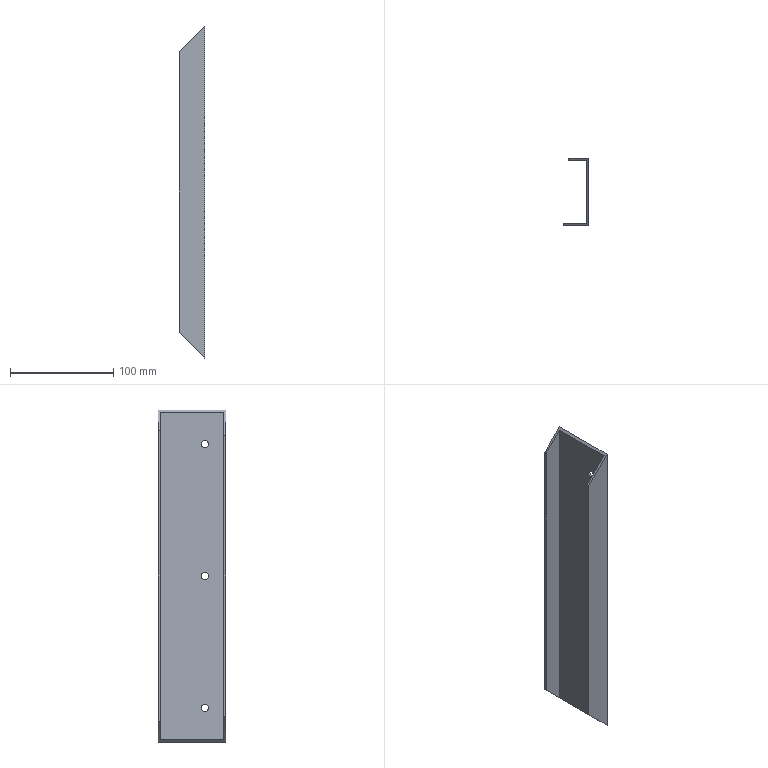Part | STEP file | 1519D1D2-5.stp.STEP | 1 solid | 16 faces | box 25 x 65 x 321 mm | volume 65527 mm3 | plane 10 | cylinder 6 | commonest cylinder face diameters 7 x6
STEP:
#1=CARTESIAN_POINT('',(-25.,0.,135.5));
#2=VERTEX_POINT('',#1);
#3=CARTESIAN_POINT('',(0.,0.,160.5));
#4=VERTEX_POINT('',#3);
#5=CARTESIAN_POINT('',(-25.,0.,135.5));
#6=DIRECTION('',(0.7071,0.,0.7071));
#7=VECTOR('',#6,1000.);
#8=LINE('',#5,#7);
#9=EDGE_CURVE('',#2,#4,#8,.T.);
#10=ORIENTED_EDGE('',*,*,#9,.F.);
#11=CARTESIAN_POINT('',(-25.,0.,-135.5));
#12=VERTEX_POINT('',#11);
#13=CARTESIAN_POINT('',(-25.,0.,-135.5));
#14=DIRECTION('',(0.,0.,1.));
#15=VECTOR('',#14,1000.);
#16=LINE('',#13,#15);
#17=EDGE_CURVE('',#12,#2,#16,.T.);
#18=ORIENTED_EDGE('',*,*,#17,.F.);
#19=CARTESIAN_POINT('',(0.,0.,-160.5));
#20=VERTEX_POINT('',#19);
#21=CARTESIAN_POINT('',(-25.,0.,-135.5));
#22=DIRECTION('',(0.7071,0.,-0.7071));
#23=VECTOR('',#22,1000.);
#24=LINE('',#21,#23);
#25=EDGE_CURVE('',#12,#20,#24,.T.);
#26=ORIENTED_EDGE('',*,*,#25,.T.);
#27=CARTESIAN_POINT('',(0.,0.,-160.5));
#28=DIRECTION('',(0.,0.,1.));
#29=VECTOR('',#28,1000.);
#30=LINE('',#27,#29);
#31=EDGE_CURVE('',#20,#4,#30,.T.);
#32=ORIENTED_EDGE('',*,*,#31,.T.);
#33=EDGE_LOOP('',(#10,#18,#26,#32));
#34=FACE_OUTER_BOUND('',#33,.T.);
#35=CARTESIAN_POINT('',(-25.,0.,-160.5));
#36=DIRECTION('',(0.,-1.,0.));
#37=DIRECTION('',(0.,0.,-1.));
#38=AXIS2_PLACEMENT_3D('',#35,#36,#37);
#39=PLANE('',#38);
#40=ADVANCED_FACE('',(#34),#39,.T.);
#41=CARTESIAN_POINT('',(0.,20.,-131.));
#42=VERTEX_POINT('',#41);
#43=CARTESIAN_POINT('',(0.,20.,-124.));
#44=VERTEX_POINT('',#43);
#45=CARTESIAN_POINT('',(0.,20.,-127.5));
#46=DIRECTION('',(1.,0.,0.));
#47=DIRECTION('',(0.,0.,-1.));
#48=AXIS2_PLACEMENT_3D('',#45,#46,#47);
#49=CIRCLE('',#48,3.5);
#50=EDGE_CURVE('',#42,#44,#49,.T.);
#51=ORIENTED_EDGE('',*,*,#50,.F.);
#52=CARTESIAN_POINT('',(0.,20.,-127.5));
#53=DIRECTION('',(1.,0.,0.));
#54=DIRECTION('',(0.,0.,1.));
#55=AXIS2_PLACEMENT_3D('',#52,#53,#54);
#56=CIRCLE('',#55,3.5);
#57=EDGE_CURVE('',#44,#42,#56,.T.);
#58=ORIENTED_EDGE('',*,*,#57,.F.);
#59=EDGE_LOOP('',(#51,#58));
#60=FACE_BOUND('',#59,.T.);
#61=CARTESIAN_POINT('',(0.,20.,-3.5));
#62=VERTEX_POINT('',#61);
#63=CARTESIAN_POINT('',(0.,20.,3.5));
#64=VERTEX_POINT('',#63);
#65=CARTESIAN_POINT('',(0.,20.,0.));
#66=DIRECTION('',(1.,0.,0.));
#67=DIRECTION('',(0.,0.,-1.));
#68=AXIS2_PLACEMENT_3D('',#65,#66,#67);
#69=CIRCLE('',#68,3.5);
#70=EDGE_CURVE('',#62,#64,#69,.T.);
#71=ORIENTED_EDGE('',*,*,#70,.F.);
#72=CARTESIAN_POINT('',(0.,20.,0.));
#73=DIRECTION('',(1.,0.,0.));
#74=DIRECTION('',(0.,0.,1.));
#75=AXIS2_PLACEMENT_3D('',#72,#73,#74);
#76=CIRCLE('',#75,3.5);
#77=EDGE_CURVE('',#64,#62,#76,.T.);
#78=ORIENTED_EDGE('',*,*,#77,.F.);
#79=EDGE_LOOP('',(#71,#78));
#80=FACE_BOUND('',#79,.T.);
#81=CARTESIAN_POINT('',(0.,20.,124.));
#82=VERTEX_POINT('',#81);
#83=CARTESIAN_POINT('',(0.,20.,131.));
#84=VERTEX_POINT('',#83);
#85=CARTESIAN_POINT('',(0.,20.,127.5));
#86=DIRECTION('',(1.,0.,0.));
#87=DIRECTION('',(0.,0.,-1.));
#88=AXIS2_PLACEMENT_3D('',#85,#86,#87);
#89=CIRCLE('',#88,3.5);
#90=EDGE_CURVE('',#82,#84,#89,.T.);
#91=ORIENTED_EDGE('',*,*,#90,.F.);
#92=CARTESIAN_POINT('',(0.,20.,127.5));
#93=DIRECTION('',(1.,0.,0.));
#94=DIRECTION('',(0.,0.,1.));
#95=AXIS2_PLACEMENT_3D('',#92,#93,#94);
#96=CIRCLE('',#95,3.5);
#97=EDGE_CURVE('',#84,#82,#96,.T.);
#98=ORIENTED_EDGE('',*,*,#97,.F.);
#99=EDGE_LOOP('',(#91,#98));
#100=FACE_BOUND('',#99,.T.);
#101=CARTESIAN_POINT('',(0.,65.,-160.5));
#102=VERTEX_POINT('',#101);
#103=CARTESIAN_POINT('',(0.,65.,-160.5));
#104=DIRECTION('',(0.,-1.,0.));
#105=VECTOR('',#104,1000.);
#106=LINE('',#103,#105);
#107=EDGE_CURVE('',#102,#20,#106,.T.);
#108=ORIENTED_EDGE('',*,*,#107,.F.);
#109=CARTESIAN_POINT('',(0.,65.,160.5));
#110=VERTEX_POINT('',#109);
#111=CARTESIAN_POINT('',(0.,65.,-160.5));
#112=DIRECTION('',(0.,0.,1.));
#113=VECTOR('',#112,1000.);
#114=LINE('',#111,#113);
#115=EDGE_CURVE('',#102,#110,#114,.T.);
#116=ORIENTED_EDGE('',*,*,#115,.T.);
#117=CARTESIAN_POINT('',(0.,65.,160.5));
#118=DIRECTION('',(0.,-1.,0.));
#119=VECTOR('',#118,1000.);
#120=LINE('',#117,#119);
#121=EDGE_CURVE('',#110,#4,#120,.T.);
#122=ORIENTED_EDGE('',*,*,#121,.T.);
#123=ORIENTED_EDGE('',*,*,#31,.F.);
#124=EDGE_LOOP('',(#108,#116,#122,#123));
#125=FACE_OUTER_BOUND('',#124,.T.);
#126=CARTESIAN_POINT('',(0.,0.,-160.5));
#127=DIRECTION('',(1.,0.,0.));
#128=DIRECTION('',(0.,1.,0.));
#129=AXIS2_PLACEMENT_3D('',#126,#127,#128);
#130=PLANE('',#129);
#131=ADVANCED_FACE('',(#60,#80,#100,#125),#130,.T.);
#132=ORIENTED_EDGE('',*,*,#121,.F.);
#133=CARTESIAN_POINT('',(-20.,65.,140.5));
#134=VERTEX_POINT('',#133);
#135=CARTESIAN_POINT('',(0.,65.,160.5));
#136=DIRECTION('',(-0.7071,0.,-0.7071));
#137=VECTOR('',#136,1000.);
#138=LINE('',#135,#137);
#139=EDGE_CURVE('',#110,#134,#138,.T.);
#140=ORIENTED_EDGE('',*,*,#139,.T.);
#141=CARTESIAN_POINT('',(-20.,63.,140.5));
#142=VERTEX_POINT('',#141);
#143=CARTESIAN_POINT('',(-20.,65.,140.5));
#144=DIRECTION('',(0.,-1.,0.));
#145=VECTOR('',#144,1000.);
#146=LINE('',#143,#145);
#147=EDGE_CURVE('',#134,#142,#146,.T.);
#148=ORIENTED_EDGE('',*,*,#147,.T.);
#149=CARTESIAN_POINT('',(-2.,63.,158.5));
#150=VERTEX_POINT('',#149);
#151=CARTESIAN_POINT('',(-2.,63.,158.5));
#152=DIRECTION('',(-0.7071,0.,-0.7071));
#153=VECTOR('',#152,1000.);
#154=LINE('',#151,#153);
#155=EDGE_CURVE('',#150,#142,#154,.T.);
#156=ORIENTED_EDGE('',*,*,#155,.F.);
#157=CARTESIAN_POINT('',(-2.,2.,158.5));
#158=VERTEX_POINT('',#157);
#159=CARTESIAN_POINT('',(-2.,63.,158.5));
#160=DIRECTION('',(0.,-1.,0.));
#161=VECTOR('',#160,1000.);
#162=LINE('',#159,#161);
#163=EDGE_CURVE('',#150,#158,#162,.T.);
#164=ORIENTED_EDGE('',*,*,#163,.T.);
#165=CARTESIAN_POINT('',(-25.,2.,135.5));
#166=VERTEX_POINT('',#165);
#167=CARTESIAN_POINT('',(-2.,2.,158.5));
#168=DIRECTION('',(-0.7071,0.,-0.7071));
#169=VECTOR('',#168,1000.);
#170=LINE('',#167,#169);
#171=EDGE_CURVE('',#158,#166,#170,.T.);
#172=ORIENTED_EDGE('',*,*,#171,.T.);
#173=CARTESIAN_POINT('',(-25.,2.,135.5));
#174=DIRECTION('',(0.,-1.,0.));
#175=VECTOR('',#174,1000.);
#176=LINE('',#173,#175);
#177=EDGE_CURVE('',#166,#2,#176,.T.);
#178=ORIENTED_EDGE('',*,*,#177,.T.);
#179=ORIENTED_EDGE('',*,*,#9,.T.);
#180=EDGE_LOOP('',(#132,#140,#148,#156,#164,#172,#178,#179));
#181=FACE_OUTER_BOUND('',#180,.T.);
#182=CARTESIAN_POINT('',(0.,65.,160.5));
#183=DIRECTION('',(0.7071,0.,-0.7071));
#184=DIRECTION('',(0.,-1.,0.));
#185=AXIS2_PLACEMENT_3D('',#182,#183,#184);
#186=PLANE('',#185);
#187=ADVANCED_FACE('',(#181),#186,.F.);
#188=ORIENTED_EDGE('',*,*,#17,.T.);
#189=ORIENTED_EDGE('',*,*,#177,.F.);
#190=CARTESIAN_POINT('',(-25.,2.,-135.5));
#191=VERTEX_POINT('',#190);
#192=CARTESIAN_POINT('',(-25.,2.,-135.5));
#193=DIRECTION('',(0.,0.,1.));
#194=VECTOR('',#193,1000.);
#195=LINE('',#192,#194);
#196=EDGE_CURVE('',#191,#166,#195,.T.);
#197=ORIENTED_EDGE('',*,*,#196,.F.);
#198=CARTESIAN_POINT('',(-25.,2.,-135.5));
#199=DIRECTION('',(0.,-1.,0.));
#200=VECTOR('',#199,1000.);
#201=LINE('',#198,#200);
#202=EDGE_CURVE('',#191,#12,#201,.T.);
#203=ORIENTED_EDGE('',*,*,#202,.T.);
#204=EDGE_LOOP('',(#188,#189,#197,#203));
#205=FACE_OUTER_BOUND('',#204,.T.);
#206=CARTESIAN_POINT('',(-25.,2.,-160.5));
#207=DIRECTION('',(-1.,0.,0.));
#208=DIRECTION('',(0.,0.,1.));
#209=AXIS2_PLACEMENT_3D('',#206,#207,#208);
#210=PLANE('',#209);
#211=ADVANCED_FACE('',(#205),#210,.T.);
#212=CARTESIAN_POINT('',(-20.,65.,-140.5));
#213=VERTEX_POINT('',#212);
#214=CARTESIAN_POINT('',(-20.,65.,-140.5));
#215=DIRECTION('',(0.7071,0.,-0.7071));
#216=VECTOR('',#215,1000.);
#217=LINE('',#214,#216);
#218=EDGE_CURVE('',#213,#102,#217,.T.);
#219=ORIENTED_EDGE('',*,*,#218,.T.);
#220=ORIENTED_EDGE('',*,*,#107,.T.);
#221=ORIENTED_EDGE('',*,*,#25,.F.);
#222=ORIENTED_EDGE('',*,*,#202,.F.);
#223=CARTESIAN_POINT('',(-2.,2.,-158.5));
#224=VERTEX_POINT('',#223);
#225=CARTESIAN_POINT('',(-2.,2.,-158.5));
#226=DIRECTION('',(-0.7071,0.,0.7071));
#227=VECTOR('',#226,1000.);
#228=LINE('',#225,#227);
#229=EDGE_CURVE('',#224,#191,#228,.T.);
#230=ORIENTED_EDGE('',*,*,#229,.F.);
#231=CARTESIAN_POINT('',(-2.,63.,-158.5));
#232=VERTEX_POINT('',#231);
#233=CARTESIAN_POINT('',(-2.,63.,-158.5));
#234=DIRECTION('',(0.,-1.,0.));
#235=VECTOR('',#234,1000.);
#236=LINE('',#233,#235);
#237=EDGE_CURVE('',#232,#224,#236,.T.);
#238=ORIENTED_EDGE('',*,*,#237,.F.);
#239=CARTESIAN_POINT('',(-20.,63.,-140.5));
#240=VERTEX_POINT('',#239);
#241=CARTESIAN_POINT('',(-2.,63.,-158.5));
#242=DIRECTION('',(-0.7071,0.,0.7071));
#243=VECTOR('',#242,1000.);
#244=LINE('',#241,#243);
#245=EDGE_CURVE('',#232,#240,#244,.T.);
#246=ORIENTED_EDGE('',*,*,#245,.T.);
#247=CARTESIAN_POINT('',(-20.,65.,-140.5));
#248=DIRECTION('',(0.,-1.,0.));
#249=VECTOR('',#248,1000.);
#250=LINE('',#247,#249);
#251=EDGE_CURVE('',#213,#240,#250,.T.);
#252=ORIENTED_EDGE('',*,*,#251,.F.);
#253=EDGE_LOOP('',(#219,#220,#221,#222,#230,#238,#246,#252));
#254=FACE_OUTER_BOUND('',#253,.T.);
#255=CARTESIAN_POINT('',(-50.,65.,-110.5));
#256=DIRECTION('',(0.7071,0.,0.7071));
#257=DIRECTION('',(0.,-1.,0.));
#258=AXIS2_PLACEMENT_3D('',#255,#256,#257);
#259=PLANE('',#258);
#260=ADVANCED_FACE('',(#254),#259,.F.);
#261=CARTESIAN_POINT('',(-20.,63.,-140.5));
#262=DIRECTION('',(0.,0.,1.));
#263=VECTOR('',#262,1000.);
#264=LINE('',#261,#263);
#265=EDGE_CURVE('',#240,#142,#264,.T.);
#266=ORIENTED_EDGE('',*,*,#265,.T.);
#267=ORIENTED_EDGE('',*,*,#147,.F.);
#268=CARTESIAN_POINT('',(-20.,65.,-140.5));
#269=DIRECTION('',(0.,0.,1.));
#270=VECTOR('',#269,1000.);
#271=LINE('',#268,#270);
#272=EDGE_CURVE('',#213,#134,#271,.T.);
#273=ORIENTED_EDGE('',*,*,#272,.F.);
#274=ORIENTED_EDGE('',*,*,#251,.T.);
#275=EDGE_LOOP('',(#266,#267,#273,#274));
#276=FACE_OUTER_BOUND('',#275,.T.);
#277=CARTESIAN_POINT('',(-20.,65.,-160.5));
#278=DIRECTION('',(-1.,0.,0.));
#279=DIRECTION('',(0.,0.,1.));
#280=AXIS2_PLACEMENT_3D('',#277,#278,#279);
#281=PLANE('',#280);
#282=ADVANCED_FACE('',(#276),#281,.T.);
#283=ORIENTED_EDGE('',*,*,#272,.T.);
#284=ORIENTED_EDGE('',*,*,#139,.F.);
#285=ORIENTED_EDGE('',*,*,#115,.F.);
#286=ORIENTED_EDGE('',*,*,#218,.F.);
#287=EDGE_LOOP('',(#283,#284,#285,#286));
#288=FACE_OUTER_BOUND('',#287,.T.);
#289=CARTESIAN_POINT('',(0.,65.,-160.5));
#290=DIRECTION('',(0.,1.,0.));
#291=DIRECTION('',(1.,0.,0.));
#292=AXIS2_PLACEMENT_3D('',#289,#290,#291);
#293=PLANE('',#292);
#294=ADVANCED_FACE('',(#288),#293,.T.);
#295=CARTESIAN_POINT('',(-2.,63.,-158.5));
#296=DIRECTION('',(0.,0.,1.));
#297=VECTOR('',#296,1000.);
#298=LINE('',#295,#297);
#299=EDGE_CURVE('',#232,#150,#298,.T.);
#300=ORIENTED_EDGE('',*,*,#299,.T.);
#301=ORIENTED_EDGE('',*,*,#155,.T.);
#302=ORIENTED_EDGE('',*,*,#265,.F.);
#303=ORIENTED_EDGE('',*,*,#245,.F.);
#304=EDGE_LOOP('',(#300,#301,#302,#303));
#305=FACE_OUTER_BOUND('',#304,.T.);
#306=CARTESIAN_POINT('',(-20.,63.,-160.5));
#307=DIRECTION('',(0.,-1.,0.));
#308=DIRECTION('',(0.,0.,-1.));
#309=AXIS2_PLACEMENT_3D('',#306,#307,#308);
#310=PLANE('',#309);
#311=ADVANCED_FACE('',(#305),#310,.T.);
#312=CARTESIAN_POINT('',(-2.,20.,-131.));
#313=VERTEX_POINT('',#312);
#314=CARTESIAN_POINT('',(-2.,20.,-124.));
#315=VERTEX_POINT('',#314);
#316=CARTESIAN_POINT('',(-2.,20.,-127.5));
#317=DIRECTION('',(1.,0.,0.));
#318=DIRECTION('',(0.,0.,-1.));
#319=AXIS2_PLACEMENT_3D('',#316,#317,#318);
#320=CIRCLE('',#319,3.5);
#321=EDGE_CURVE('',#313,#315,#320,.T.);
#322=ORIENTED_EDGE('',*,*,#321,.T.);
#323=CARTESIAN_POINT('',(-2.,20.,-127.5));
#324=DIRECTION('',(1.,0.,0.));
#325=DIRECTION('',(0.,0.,1.));
#326=AXIS2_PLACEMENT_3D('',#323,#324,#325);
#327=CIRCLE('',#326,3.5);
#328=EDGE_CURVE('',#315,#313,#327,.T.);
#329=ORIENTED_EDGE('',*,*,#328,.T.);
#330=EDGE_LOOP('',(#322,#329));
#331=FACE_BOUND('',#330,.T.);
#332=CARTESIAN_POINT('',(-2.,20.,-3.5));
#333=VERTEX_POINT('',#332);
#334=CARTESIAN_POINT('',(-2.,20.,3.5));
#335=VERTEX_POINT('',#334);
#336=CARTESIAN_POINT('',(-2.,20.,0.));
#337=DIRECTION('',(1.,0.,0.));
#338=DIRECTION('',(0.,0.,-1.));
#339=AXIS2_PLACEMENT_3D('',#336,#337,#338);
#340=CIRCLE('',#339,3.5);
#341=EDGE_CURVE('',#333,#335,#340,.T.);
#342=ORIENTED_EDGE('',*,*,#341,.T.);
#343=CARTESIAN_POINT('',(-2.,20.,0.));
#344=DIRECTION('',(1.,0.,0.));
#345=DIRECTION('',(0.,0.,1.));
#346=AXIS2_PLACEMENT_3D('',#343,#344,#345);
#347=CIRCLE('',#346,3.5);
#348=EDGE_CURVE('',#335,#333,#347,.T.);
#349=ORIENTED_EDGE('',*,*,#348,.T.);
#350=EDGE_LOOP('',(#342,#349));
#351=FACE_BOUND('',#350,.T.);
#352=CARTESIAN_POINT('',(-2.,20.,124.));
#353=VERTEX_POINT('',#352);
#354=CARTESIAN_POINT('',(-2.,20.,131.));
#355=VERTEX_POINT('',#354);
#356=CARTESIAN_POINT('',(-2.,20.,127.5));
#357=DIRECTION('',(1.,0.,0.));
#358=DIRECTION('',(0.,0.,-1.));
#359=AXIS2_PLACEMENT_3D('',#356,#357,#358);
#360=CIRCLE('',#359,3.5);
#361=EDGE_CURVE('',#353,#355,#360,.T.);
#362=ORIENTED_EDGE('',*,*,#361,.T.);
#363=CARTESIAN_POINT('',(-2.,20.,127.5));
#364=DIRECTION('',(1.,0.,0.));
#365=DIRECTION('',(0.,0.,1.));
#366=AXIS2_PLACEMENT_3D('',#363,#364,#365);
#367=CIRCLE('',#366,3.5);
#368=EDGE_CURVE('',#355,#353,#367,.T.);
#369=ORIENTED_EDGE('',*,*,#368,.T.);
#370=EDGE_LOOP('',(#362,#369));
#371=FACE_BOUND('',#370,.T.);
#372=CARTESIAN_POINT('',(-2.,2.,-158.5));
#373=DIRECTION('',(0.,0.,1.));
#374=VECTOR('',#373,1000.);
#375=LINE('',#372,#374);
#376=EDGE_CURVE('',#224,#158,#375,.T.);
#377=ORIENTED_EDGE('',*,*,#376,.T.);
#378=ORIENTED_EDGE('',*,*,#163,.F.);
#379=ORIENTED_EDGE('',*,*,#299,.F.);
#380=ORIENTED_EDGE('',*,*,#237,.T.);
#381=EDGE_LOOP('',(#377,#378,#379,#380));
#382=FACE_OUTER_BOUND('',#381,.T.);
#383=CARTESIAN_POINT('',(-2.,63.,-160.5));
#384=DIRECTION('',(-1.,0.,0.));
#385=DIRECTION('',(0.,0.,1.));
#386=AXIS2_PLACEMENT_3D('',#383,#384,#385);
#387=PLANE('',#386);
#388=ADVANCED_FACE('',(#331,#351,#371,#382),#387,.T.);
#389=ORIENTED_EDGE('',*,*,#196,.T.);
#390=ORIENTED_EDGE('',*,*,#171,.F.);
#391=ORIENTED_EDGE('',*,*,#376,.F.);
#392=ORIENTED_EDGE('',*,*,#229,.T.);
#393=EDGE_LOOP('',(#389,#390,#391,#392));
#394=FACE_OUTER_BOUND('',#393,.T.);
#395=CARTESIAN_POINT('',(-2.,2.,-160.5));
#396=DIRECTION('',(0.,1.,0.));
#397=DIRECTION('',(1.,0.,0.));
#398=AXIS2_PLACEMENT_3D('',#395,#396,#397);
#399=PLANE('',#398);
#400=ADVANCED_FACE('',(#394),#399,.T.);
#401=CARTESIAN_POINT('',(0.,20.,-131.));
#402=DIRECTION('',(-1.,0.,0.));
#403=VECTOR('',#402,1000.);
#404=LINE('',#401,#403);
#405=EDGE_CURVE('',#42,#313,#404,.T.);
#406=ORIENTED_EDGE('',*,*,#405,.T.);
#407=ORIENTED_EDGE('',*,*,#328,.F.);
#408=CARTESIAN_POINT('',(0.,20.,-124.));
#409=DIRECTION('',(-1.,0.,0.));
#410=VECTOR('',#409,1000.);
#411=LINE('',#408,#410);
#412=EDGE_CURVE('',#44,#315,#411,.T.);
#413=ORIENTED_EDGE('',*,*,#412,.F.);
#414=ORIENTED_EDGE('',*,*,#57,.T.);
#415=EDGE_LOOP('',(#406,#407,#413,#414));
#416=FACE_OUTER_BOUND('',#415,.T.);
#417=CARTESIAN_POINT('',(0.,20.,-127.5));
#418=DIRECTION('',(1.,0.,0.));
#419=DIRECTION('',(0.,0.,1.));
#420=AXIS2_PLACEMENT_3D('',#417,#418,#419);
#421=CYLINDRICAL_SURFACE('',#420,3.5);
#422=ADVANCED_FACE('',(#416),#421,.F.);
#423=ORIENTED_EDGE('',*,*,#412,.T.);
#424=ORIENTED_EDGE('',*,*,#321,.F.);
#425=ORIENTED_EDGE('',*,*,#405,.F.);
#426=ORIENTED_EDGE('',*,*,#50,.T.);
#427=EDGE_LOOP('',(#423,#424,#425,#426));
#428=FACE_OUTER_BOUND('',#427,.T.);
#429=CARTESIAN_POINT('',(0.,20.,-127.5));
#430=DIRECTION('',(1.,0.,0.));
#431=DIRECTION('',(0.,0.,1.));
#432=AXIS2_PLACEMENT_3D('',#429,#430,#431);
#433=CYLINDRICAL_SURFACE('',#432,3.5);
#434=ADVANCED_FACE('',(#428),#433,.F.);
#435=CARTESIAN_POINT('',(0.,20.,-3.5));
#436=DIRECTION('',(-1.,0.,0.));
#437=VECTOR('',#436,1000.);
#438=LINE('',#435,#437);
#439=EDGE_CURVE('',#62,#333,#438,.T.);
#440=ORIENTED_EDGE('',*,*,#439,.T.);
#441=ORIENTED_EDGE('',*,*,#348,.F.);
#442=CARTESIAN_POINT('',(0.,20.,3.5));
#443=DIRECTION('',(-1.,0.,0.));
#444=VECTOR('',#443,1000.);
#445=LINE('',#442,#444);
#446=EDGE_CURVE('',#64,#335,#445,.T.);
#447=ORIENTED_EDGE('',*,*,#446,.F.);
#448=ORIENTED_EDGE('',*,*,#77,.T.);
#449=EDGE_LOOP('',(#440,#441,#447,#448));
#450=FACE_OUTER_BOUND('',#449,.T.);
#451=CARTESIAN_POINT('',(0.,20.,0.));
#452=DIRECTION('',(1.,0.,0.));
#453=DIRECTION('',(0.,0.,1.));
#454=AXIS2_PLACEMENT_3D('',#451,#452,#453);
#455=CYLINDRICAL_SURFACE('',#454,3.5);
#456=ADVANCED_FACE('',(#450),#455,.F.);
#457=ORIENTED_EDGE('',*,*,#446,.T.);
#458=ORIENTED_EDGE('',*,*,#341,.F.);
#459=ORIENTED_EDGE('',*,*,#439,.F.);
#460=ORIENTED_EDGE('',*,*,#70,.T.);
#461=EDGE_LOOP('',(#457,#458,#459,#460));
#462=FACE_OUTER_BOUND('',#461,.T.);
#463=CARTESIAN_POINT('',(0.,20.,0.));
#464=DIRECTION('',(1.,0.,0.));
#465=DIRECTION('',(0.,0.,1.));
#466=AXIS2_PLACEMENT_3D('',#463,#464,#465);
#467=CYLINDRICAL_SURFACE('',#466,3.5);
#468=ADVANCED_FACE('',(#462),#467,.F.);
#469=CARTESIAN_POINT('',(0.,20.,124.));
#470=DIRECTION('',(-1.,0.,0.));
#471=VECTOR('',#470,1000.);
#472=LINE('',#469,#471);
#473=EDGE_CURVE('',#82,#353,#472,.T.);
#474=ORIENTED_EDGE('',*,*,#473,.T.);
#475=ORIENTED_EDGE('',*,*,#368,.F.);
#476=CARTESIAN_POINT('',(0.,20.,131.));
#477=DIRECTION('',(-1.,0.,0.));
#478=VECTOR('',#477,1000.);
#479=LINE('',#476,#478);
#480=EDGE_CURVE('',#84,#355,#479,.T.);
#481=ORIENTED_EDGE('',*,*,#480,.F.);
#482=ORIENTED_EDGE('',*,*,#97,.T.);
#483=EDGE_LOOP('',(#474,#475,#481,#482));
#484=FACE_OUTER_BOUND('',#483,.T.);
#485=CARTESIAN_POINT('',(0.,20.,127.5));
#486=DIRECTION('',(1.,0.,0.));
#487=DIRECTION('',(0.,0.,1.));
#488=AXIS2_PLACEMENT_3D('',#485,#486,#487);
#489=CYLINDRICAL_SURFACE('',#488,3.5);
#490=ADVANCED_FACE('',(#484),#489,.F.);
#491=ORIENTED_EDGE('',*,*,#480,.T.);
#492=ORIENTED_EDGE('',*,*,#361,.F.);
#493=ORIENTED_EDGE('',*,*,#473,.F.);
#494=ORIENTED_EDGE('',*,*,#90,.T.);
#495=EDGE_LOOP('',(#491,#492,#493,#494));
#496=FACE_OUTER_BOUND('',#495,.T.);
#497=CARTESIAN_POINT('',(0.,20.,127.5));
#498=DIRECTION('',(1.,0.,0.));
#499=DIRECTION('',(0.,0.,1.));
#500=AXIS2_PLACEMENT_3D('',#497,#498,#499);
#501=CYLINDRICAL_SURFACE('',#500,3.5);
#502=ADVANCED_FACE('',(#496),#501,.F.);
#503=CLOSED_SHELL('',(#40,#131,#187,#211,#260,#282,#294,#311,#388,#400,#422,#434,#456,#468,#490,#502));
#504=MANIFOLD_SOLID_BREP('',#503);
#505=CARTESIAN_POINT('',(0.,0.,0.));
#506=DIRECTION('',(0.,0.,1.));
#507=DIRECTION('',(1.,0.,0.));
#508=AXIS2_PLACEMENT_3D('',#505,#506,#507);
#509=(LENGTH_UNIT()NAMED_UNIT(*)SI_UNIT(.MILLI.,.METRE.));
#510=UNCERTAINTY_MEASURE_WITH_UNIT(LENGTH_MEASURE(0.00001),#509,'','');
#511=(NAMED_UNIT(*)PLANE_ANGLE_UNIT()SI_UNIT($,.RADIAN.));
#512=(NAMED_UNIT(*)SI_UNIT($,.STERADIAN.)SOLID_ANGLE_UNIT());
#513=(GEOMETRIC_REPRESENTATION_CONTEXT(3)GLOBAL_UNCERTAINTY_ASSIGNED_CONTEXT((#510))GLOBAL_UNIT_ASSIGNED_CONTEXT((#509,#511,#512))REPRESENTATION_CONTEXT('',''));
#514=ADVANCED_BREP_SHAPE_REPRESENTATION('',(#504,#508),#513);